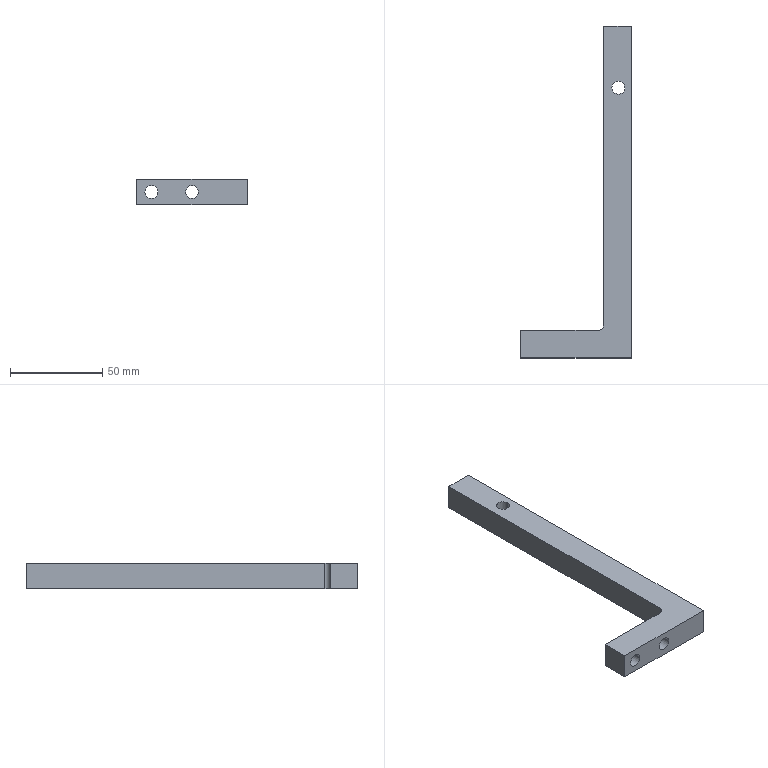Part | SolidWorks | features Cut 1, Extrusion 1, Fillet 1, ICE 1 | 1 solid | 15 faces | box 60 x 180 x 14 mm | volume 45584 mm3 | plane 8 | cylinder 7 | commonest cylinder face diameters 7 x6 6 x1
STEP:
#1=CARTESIAN_POINT('',(-10.5,146.5,7.));
#2=VERTEX_POINT('',#1);
#3=CARTESIAN_POINT('',(-3.5,146.5,7.));
#4=VERTEX_POINT('',#3);
#5=CARTESIAN_POINT('',(-7.,146.5,7.));
#6=DIRECTION('',(0.,0.,1.));
#7=DIRECTION('',(-1.,0.,0.));
#8=AXIS2_PLACEMENT_3D('',#5,#6,#7);
#9=CIRCLE('',#8,3.5);
#10=EDGE_CURVE('',#2,#4,#9,.T.);
#11=ORIENTED_EDGE('',*,*,#10,.T.);
#12=CARTESIAN_POINT('',(-3.5,146.5,-7.));
#13=VERTEX_POINT('',#12);
#14=CARTESIAN_POINT('',(-3.5,146.5,7.001));
#15=DIRECTION('',(0.,0.,-1.));
#16=VECTOR('',#15,1000.);
#17=LINE('',#14,#16);
#18=EDGE_CURVE('',#4,#13,#17,.T.);
#19=ORIENTED_EDGE('',*,*,#18,.T.);
#20=CARTESIAN_POINT('',(-10.5,146.5,-7.));
#21=VERTEX_POINT('',#20);
#22=CARTESIAN_POINT('',(-7.,146.5,-7.));
#23=DIRECTION('',(0.,0.,-1.));
#24=DIRECTION('',(-1.,0.,0.));
#25=AXIS2_PLACEMENT_3D('',#22,#23,#24);
#26=CIRCLE('',#25,3.5);
#27=EDGE_CURVE('',#13,#21,#26,.T.);
#28=ORIENTED_EDGE('',*,*,#27,.T.);
#29=CARTESIAN_POINT('',(-10.5,146.5,7.001));
#30=DIRECTION('',(0.,0.,-1.));
#31=VECTOR('',#30,1000.);
#32=LINE('',#29,#31);
#33=EDGE_CURVE('',#2,#21,#32,.T.);
#34=ORIENTED_EDGE('',*,*,#33,.F.);
#35=EDGE_LOOP('',(#11,#19,#28,#34));
#36=FACE_OUTER_BOUND('',#35,.T.);
#37=CARTESIAN_POINT('',(-7.,146.5,7.001));
#38=DIRECTION('',(0.,0.,-1.));
#39=DIRECTION('',(-1.,0.,0.));
#40=AXIS2_PLACEMENT_3D('',#37,#38,#39);
#41=CYLINDRICAL_SURFACE('',#40,3.5);
#42=ADVANCED_FACE('',(#36),#41,.F.);
#43=CARTESIAN_POINT('',(-55.5,0.,0.));
#44=VERTEX_POINT('',#43);
#45=CARTESIAN_POINT('',(-48.5,0.,0.));
#46=VERTEX_POINT('',#45);
#47=CARTESIAN_POINT('',(-52.,0.,0.));
#48=DIRECTION('',(0.,-1.,0.));
#49=DIRECTION('',(0.,0.,1.));
#50=AXIS2_PLACEMENT_3D('',#47,#48,#49);
#51=CIRCLE('',#50,3.5);
#52=EDGE_CURVE('',#44,#46,#51,.T.);
#53=ORIENTED_EDGE('',*,*,#52,.T.);
#54=CARTESIAN_POINT('',(-48.5,15.,0.));
#55=VERTEX_POINT('',#54);
#56=CARTESIAN_POINT('',(-48.5,-0.001,0.));
#57=DIRECTION('',(0.,1.,0.));
#58=VECTOR('',#57,1000.);
#59=LINE('',#56,#58);
#60=EDGE_CURVE('',#46,#55,#59,.T.);
#61=ORIENTED_EDGE('',*,*,#60,.T.);
#62=CARTESIAN_POINT('',(-55.5,15.,0.));
#63=VERTEX_POINT('',#62);
#64=CARTESIAN_POINT('',(-52.,15.,0.));
#65=DIRECTION('',(0.,1.,0.));
#66=DIRECTION('',(-1.,0.,0.));
#67=AXIS2_PLACEMENT_3D('',#64,#65,#66);
#68=CIRCLE('',#67,3.5);
#69=EDGE_CURVE('',#55,#63,#68,.T.);
#70=ORIENTED_EDGE('',*,*,#69,.T.);
#71=CARTESIAN_POINT('',(-55.5,-0.001,0.));
#72=DIRECTION('',(0.,1.,0.));
#73=VECTOR('',#72,1000.);
#74=LINE('',#71,#73);
#75=EDGE_CURVE('',#44,#63,#74,.T.);
#76=ORIENTED_EDGE('',*,*,#75,.F.);
#77=EDGE_LOOP('',(#53,#61,#70,#76));
#78=FACE_OUTER_BOUND('',#77,.T.);
#79=CARTESIAN_POINT('',(-52.,-0.001,0.));
#80=DIRECTION('',(0.,1.,0.));
#81=DIRECTION('',(-1.,0.,0.));
#82=AXIS2_PLACEMENT_3D('',#79,#80,#81);
#83=CYLINDRICAL_SURFACE('',#82,3.5);
#84=ADVANCED_FACE('',(#78),#83,.F.);
#85=CARTESIAN_POINT('',(-33.5,0.,0.));
#86=VERTEX_POINT('',#85);
#87=CARTESIAN_POINT('',(-26.5,0.,0.));
#88=VERTEX_POINT('',#87);
#89=CARTESIAN_POINT('',(-30.,0.,0.));
#90=DIRECTION('',(0.,-1.,0.));
#91=DIRECTION('',(0.,0.,1.));
#92=AXIS2_PLACEMENT_3D('',#89,#90,#91);
#93=CIRCLE('',#92,3.5);
#94=EDGE_CURVE('',#86,#88,#93,.T.);
#95=ORIENTED_EDGE('',*,*,#94,.T.);
#96=CARTESIAN_POINT('',(-26.5,15.,0.));
#97=VERTEX_POINT('',#96);
#98=CARTESIAN_POINT('',(-26.5,-0.001,0.));
#99=DIRECTION('',(0.,1.,0.));
#100=VECTOR('',#99,1000.);
#101=LINE('',#98,#100);
#102=EDGE_CURVE('',#88,#97,#101,.T.);
#103=ORIENTED_EDGE('',*,*,#102,.T.);
#104=CARTESIAN_POINT('',(-33.5,15.,0.));
#105=VERTEX_POINT('',#104);
#106=CARTESIAN_POINT('',(-30.,15.,0.));
#107=DIRECTION('',(0.,1.,0.));
#108=DIRECTION('',(-1.,0.,0.));
#109=AXIS2_PLACEMENT_3D('',#106,#107,#108);
#110=CIRCLE('',#109,3.5);
#111=EDGE_CURVE('',#97,#105,#110,.T.);
#112=ORIENTED_EDGE('',*,*,#111,.T.);
#113=CARTESIAN_POINT('',(-33.5,-0.001,0.));
#114=DIRECTION('',(0.,1.,0.));
#115=VECTOR('',#114,1000.);
#116=LINE('',#113,#115);
#117=EDGE_CURVE('',#86,#105,#116,.T.);
#118=ORIENTED_EDGE('',*,*,#117,.F.);
#119=EDGE_LOOP('',(#95,#103,#112,#118));
#120=FACE_OUTER_BOUND('',#119,.T.);
#121=CARTESIAN_POINT('',(-30.,-0.001,0.));
#122=DIRECTION('',(0.,1.,0.));
#123=DIRECTION('',(-1.,0.,0.));
#124=AXIS2_PLACEMENT_3D('',#121,#122,#123);
#125=CYLINDRICAL_SURFACE('',#124,3.5);
#126=ADVANCED_FACE('',(#120),#125,.F.);
#127=CARTESIAN_POINT('',(0.,0.,-7.));
#128=VERTEX_POINT('',#127);
#129=CARTESIAN_POINT('',(0.,180.,-7.));
#130=VERTEX_POINT('',#129);
#131=CARTESIAN_POINT('',(0.,180.,-7.));
#132=DIRECTION('',(0.,1.,0.));
#133=VECTOR('',#132,1000.);
#134=LINE('',#131,#133);
#135=EDGE_CURVE('',#128,#130,#134,.T.);
#136=ORIENTED_EDGE('',*,*,#135,.T.);
#137=CARTESIAN_POINT('',(0.,180.,7.));
#138=VERTEX_POINT('',#137);
#139=CARTESIAN_POINT('',(0.,180.,7.));
#140=DIRECTION('',(0.,0.,-1.));
#141=VECTOR('',#140,1000.);
#142=LINE('',#139,#141);
#143=EDGE_CURVE('',#138,#130,#142,.T.);
#144=ORIENTED_EDGE('',*,*,#143,.F.);
#145=CARTESIAN_POINT('',(0.,0.,7.));
#146=VERTEX_POINT('',#145);
#147=CARTESIAN_POINT('',(0.,180.,7.));
#148=DIRECTION('',(0.,1.,0.));
#149=VECTOR('',#148,1000.);
#150=LINE('',#147,#149);
#151=EDGE_CURVE('',#146,#138,#150,.T.);
#152=ORIENTED_EDGE('',*,*,#151,.F.);
#153=CARTESIAN_POINT('',(0.,0.,7.));
#154=DIRECTION('',(0.,0.,-1.));
#155=VECTOR('',#154,1000.);
#156=LINE('',#153,#155);
#157=EDGE_CURVE('',#146,#128,#156,.T.);
#158=ORIENTED_EDGE('',*,*,#157,.T.);
#159=EDGE_LOOP('',(#136,#144,#152,#158));
#160=FACE_OUTER_BOUND('',#159,.T.);
#161=CARTESIAN_POINT('',(0.,180.,7.));
#162=DIRECTION('',(-1.,0.,0.));
#163=DIRECTION('',(0.,-1.,0.));
#164=AXIS2_PLACEMENT_3D('',#161,#162,#163);
#165=PLANE('',#164);
#166=ADVANCED_FACE('',(#160),#165,.F.);
#167=CARTESIAN_POINT('',(-15.,180.,-7.));
#168=VERTEX_POINT('',#167);
#169=CARTESIAN_POINT('',(0.,180.,-7.));
#170=DIRECTION('',(-1.,0.,0.));
#171=VECTOR('',#170,1000.);
#172=LINE('',#169,#171);
#173=EDGE_CURVE('',#130,#168,#172,.T.);
#174=ORIENTED_EDGE('',*,*,#173,.T.);
#175=CARTESIAN_POINT('',(-15.,180.,7.));
#176=VERTEX_POINT('',#175);
#177=CARTESIAN_POINT('',(-15.,180.,7.));
#178=DIRECTION('',(0.,0.,-1.));
#179=VECTOR('',#178,1000.);
#180=LINE('',#177,#179);
#181=EDGE_CURVE('',#176,#168,#180,.T.);
#182=ORIENTED_EDGE('',*,*,#181,.F.);
#183=CARTESIAN_POINT('',(0.,180.,7.));
#184=DIRECTION('',(-1.,0.,0.));
#185=VECTOR('',#184,1000.);
#186=LINE('',#183,#185);
#187=EDGE_CURVE('',#138,#176,#186,.T.);
#188=ORIENTED_EDGE('',*,*,#187,.F.);
#189=ORIENTED_EDGE('',*,*,#143,.T.);
#190=EDGE_LOOP('',(#174,#182,#188,#189));
#191=FACE_OUTER_BOUND('',#190,.T.);
#192=CARTESIAN_POINT('',(0.,180.,7.));
#193=DIRECTION('',(0.,-1.,0.));
#194=DIRECTION('',(0.,0.,-1.));
#195=AXIS2_PLACEMENT_3D('',#192,#193,#194);
#196=PLANE('',#195);
#197=ADVANCED_FACE('',(#191),#196,.F.);
#198=CARTESIAN_POINT('',(-15.,18.,-7.));
#199=VERTEX_POINT('',#198);
#200=CARTESIAN_POINT('',(-15.,180.,-7.));
#201=DIRECTION('',(0.,-1.,0.));
#202=VECTOR('',#201,1000.);
#203=LINE('',#200,#202);
#204=EDGE_CURVE('',#168,#199,#203,.T.);
#205=ORIENTED_EDGE('',*,*,#204,.T.);
#206=CARTESIAN_POINT('',(-15.,18.,7.));
#207=VERTEX_POINT('',#206);
#208=CARTESIAN_POINT('',(-15.,18.,7.));
#209=DIRECTION('',(0.,0.,1.));
#210=VECTOR('',#209,1000.);
#211=LINE('',#208,#210);
#212=EDGE_CURVE('',#199,#207,#211,.T.);
#213=ORIENTED_EDGE('',*,*,#212,.T.);
#214=CARTESIAN_POINT('',(-15.,180.,7.));
#215=DIRECTION('',(0.,-1.,0.));
#216=VECTOR('',#215,1000.);
#217=LINE('',#214,#216);
#218=EDGE_CURVE('',#176,#207,#217,.T.);
#219=ORIENTED_EDGE('',*,*,#218,.F.);
#220=ORIENTED_EDGE('',*,*,#181,.T.);
#221=EDGE_LOOP('',(#205,#213,#219,#220));
#222=FACE_OUTER_BOUND('',#221,.T.);
#223=CARTESIAN_POINT('',(-15.,180.,7.));
#224=DIRECTION('',(1.,0.,0.));
#225=DIRECTION('',(0.,1.,0.));
#226=AXIS2_PLACEMENT_3D('',#223,#224,#225);
#227=PLANE('',#226);
#228=ADVANCED_FACE('',(#222),#227,.F.);
#229=CARTESIAN_POINT('',(-52.,15.,0.));
#230=DIRECTION('',(0.,1.,0.));
#231=DIRECTION('',(-1.,0.,0.));
#232=AXIS2_PLACEMENT_3D('',#229,#230,#231);
#233=CIRCLE('',#232,3.5);
#234=EDGE_CURVE('',#63,#55,#233,.T.);
#235=ORIENTED_EDGE('',*,*,#234,.F.);
#236=ORIENTED_EDGE('',*,*,#69,.F.);
#237=EDGE_LOOP('',(#235,#236));
#238=FACE_BOUND('',#237,.T.);
#239=CARTESIAN_POINT('',(-30.,15.,0.));
#240=DIRECTION('',(0.,1.,0.));
#241=DIRECTION('',(-1.,0.,0.));
#242=AXIS2_PLACEMENT_3D('',#239,#240,#241);
#243=CIRCLE('',#242,3.5);
#244=EDGE_CURVE('',#105,#97,#243,.T.);
#245=ORIENTED_EDGE('',*,*,#244,.F.);
#246=ORIENTED_EDGE('',*,*,#111,.F.);
#247=EDGE_LOOP('',(#245,#246));
#248=FACE_BOUND('',#247,.T.);
#249=CARTESIAN_POINT('',(-18.,15.,7.));
#250=VERTEX_POINT('',#249);
#251=CARTESIAN_POINT('',(-60.,15.,7.));
#252=VERTEX_POINT('',#251);
#253=CARTESIAN_POINT('',(-15.,15.,7.));
#254=DIRECTION('',(-1.,0.,0.));
#255=VECTOR('',#254,1000.);
#256=LINE('',#253,#255);
#257=EDGE_CURVE('',#250,#252,#256,.T.);
#258=ORIENTED_EDGE('',*,*,#257,.F.);
#259=CARTESIAN_POINT('',(-18.,15.,-7.));
#260=VERTEX_POINT('',#259);
#261=CARTESIAN_POINT('',(-18.,15.,-7.));
#262=DIRECTION('',(0.,0.,-1.));
#263=VECTOR('',#262,1000.);
#264=LINE('',#261,#263);
#265=EDGE_CURVE('',#250,#260,#264,.T.);
#266=ORIENTED_EDGE('',*,*,#265,.T.);
#267=CARTESIAN_POINT('',(-60.,15.,-7.));
#268=VERTEX_POINT('',#267);
#269=CARTESIAN_POINT('',(-15.,15.,-7.));
#270=DIRECTION('',(-1.,0.,0.));
#271=VECTOR('',#270,1000.);
#272=LINE('',#269,#271);
#273=EDGE_CURVE('',#260,#268,#272,.T.);
#274=ORIENTED_EDGE('',*,*,#273,.T.);
#275=CARTESIAN_POINT('',(-60.,15.,7.));
#276=DIRECTION('',(0.,0.,-1.));
#277=VECTOR('',#276,1000.);
#278=LINE('',#275,#277);
#279=EDGE_CURVE('',#252,#268,#278,.T.);
#280=ORIENTED_EDGE('',*,*,#279,.F.);
#281=EDGE_LOOP('',(#258,#266,#274,#280));
#282=FACE_OUTER_BOUND('',#281,.T.);
#283=CARTESIAN_POINT('',(-15.,15.,7.));
#284=DIRECTION('',(0.,-1.,0.));
#285=DIRECTION('',(1.,0.,0.));
#286=AXIS2_PLACEMENT_3D('',#283,#284,#285);
#287=PLANE('',#286);
#288=ADVANCED_FACE('',(#238,#248,#282),#287,.F.);
#289=CARTESIAN_POINT('',(-60.,0.,-7.));
#290=VERTEX_POINT('',#289);
#291=CARTESIAN_POINT('',(-60.,15.,-7.));
#292=DIRECTION('',(0.,-1.,0.));
#293=VECTOR('',#292,1000.);
#294=LINE('',#291,#293);
#295=EDGE_CURVE('',#268,#290,#294,.T.);
#296=ORIENTED_EDGE('',*,*,#295,.T.);
#297=CARTESIAN_POINT('',(-60.,0.,7.));
#298=VERTEX_POINT('',#297);
#299=CARTESIAN_POINT('',(-60.,0.,7.));
#300=DIRECTION('',(0.,0.,-1.));
#301=VECTOR('',#300,1000.);
#302=LINE('',#299,#301);
#303=EDGE_CURVE('',#298,#290,#302,.T.);
#304=ORIENTED_EDGE('',*,*,#303,.F.);
#305=CARTESIAN_POINT('',(-60.,15.,7.));
#306=DIRECTION('',(0.,-1.,0.));
#307=VECTOR('',#306,1000.);
#308=LINE('',#305,#307);
#309=EDGE_CURVE('',#252,#298,#308,.T.);
#310=ORIENTED_EDGE('',*,*,#309,.F.);
#311=ORIENTED_EDGE('',*,*,#279,.T.);
#312=EDGE_LOOP('',(#296,#304,#310,#311));
#313=FACE_OUTER_BOUND('',#312,.T.);
#314=CARTESIAN_POINT('',(-60.,15.,7.));
#315=DIRECTION('',(1.,0.,0.));
#316=DIRECTION('',(0.,1.,0.));
#317=AXIS2_PLACEMENT_3D('',#314,#315,#316);
#318=PLANE('',#317);
#319=ADVANCED_FACE('',(#313),#318,.F.);
#320=ORIENTED_EDGE('',*,*,#52,.F.);
#321=CARTESIAN_POINT('',(-52.,0.,0.));
#322=DIRECTION('',(0.,-1.,0.));
#323=DIRECTION('',(0.,0.,1.));
#324=AXIS2_PLACEMENT_3D('',#321,#322,#323);
#325=CIRCLE('',#324,3.5);
#326=EDGE_CURVE('',#46,#44,#325,.T.);
#327=ORIENTED_EDGE('',*,*,#326,.F.);
#328=EDGE_LOOP('',(#320,#327));
#329=FACE_BOUND('',#328,.T.);
#330=ORIENTED_EDGE('',*,*,#94,.F.);
#331=CARTESIAN_POINT('',(-30.,0.,0.));
#332=DIRECTION('',(0.,-1.,0.));
#333=DIRECTION('',(0.,0.,1.));
#334=AXIS2_PLACEMENT_3D('',#331,#332,#333);
#335=CIRCLE('',#334,3.5);
#336=EDGE_CURVE('',#88,#86,#335,.T.);
#337=ORIENTED_EDGE('',*,*,#336,.F.);
#338=EDGE_LOOP('',(#330,#337));
#339=FACE_BOUND('',#338,.T.);
#340=CARTESIAN_POINT('',(0.,0.,-7.));
#341=DIRECTION('',(1.,0.,0.));
#342=VECTOR('',#341,1000.);
#343=LINE('',#340,#342);
#344=EDGE_CURVE('',#290,#128,#343,.T.);
#345=ORIENTED_EDGE('',*,*,#344,.T.);
#346=ORIENTED_EDGE('',*,*,#157,.F.);
#347=CARTESIAN_POINT('',(0.,0.,7.));
#348=DIRECTION('',(1.,0.,0.));
#349=VECTOR('',#348,1000.);
#350=LINE('',#347,#349);
#351=EDGE_CURVE('',#298,#146,#350,.T.);
#352=ORIENTED_EDGE('',*,*,#351,.F.);
#353=ORIENTED_EDGE('',*,*,#303,.T.);
#354=EDGE_LOOP('',(#345,#346,#352,#353));
#355=FACE_OUTER_BOUND('',#354,.T.);
#356=CARTESIAN_POINT('',(0.,0.,7.));
#357=DIRECTION('',(0.,1.,0.));
#358=DIRECTION('',(0.,0.,1.));
#359=AXIS2_PLACEMENT_3D('',#356,#357,#358);
#360=PLANE('',#359);
#361=ADVANCED_FACE('',(#329,#339,#355),#360,.F.);
#362=ORIENTED_EDGE('',*,*,#10,.F.);
#363=CARTESIAN_POINT('',(-7.,146.5,7.));
#364=DIRECTION('',(0.,0.,1.));
#365=DIRECTION('',(-1.,0.,0.));
#366=AXIS2_PLACEMENT_3D('',#363,#364,#365);
#367=CIRCLE('',#366,3.5);
#368=EDGE_CURVE('',#4,#2,#367,.T.);
#369=ORIENTED_EDGE('',*,*,#368,.F.);
#370=EDGE_LOOP('',(#362,#369));
#371=FACE_BOUND('',#370,.T.);
#372=ORIENTED_EDGE('',*,*,#151,.T.);
#373=ORIENTED_EDGE('',*,*,#187,.T.);
#374=ORIENTED_EDGE('',*,*,#218,.T.);
#375=CARTESIAN_POINT('',(-18.,18.,7.));
#376=DIRECTION('',(0.,0.,-1.));
#377=DIRECTION('',(-1.,0.,0.));
#378=AXIS2_PLACEMENT_3D('',#375,#376,#377);
#379=CIRCLE('',#378,3.);
#380=EDGE_CURVE('',#207,#250,#379,.T.);
#381=ORIENTED_EDGE('',*,*,#380,.T.);
#382=ORIENTED_EDGE('',*,*,#257,.T.);
#383=ORIENTED_EDGE('',*,*,#309,.T.);
#384=ORIENTED_EDGE('',*,*,#351,.T.);
#385=EDGE_LOOP('',(#372,#373,#374,#381,#382,#383,#384));
#386=FACE_OUTER_BOUND('',#385,.T.);
#387=CARTESIAN_POINT('',(0.,0.,7.));
#388=DIRECTION('',(0.,0.,-1.));
#389=DIRECTION('',(-1.,0.,0.));
#390=AXIS2_PLACEMENT_3D('',#387,#388,#389);
#391=PLANE('',#390);
#392=ADVANCED_FACE('',(#371,#386),#391,.F.);
#393=CARTESIAN_POINT('',(-7.,146.5,-7.));
#394=DIRECTION('',(0.,0.,-1.));
#395=DIRECTION('',(-1.,0.,0.));
#396=AXIS2_PLACEMENT_3D('',#393,#394,#395);
#397=CIRCLE('',#396,3.5);
#398=EDGE_CURVE('',#21,#13,#397,.T.);
#399=ORIENTED_EDGE('',*,*,#398,.F.);
#400=ORIENTED_EDGE('',*,*,#27,.F.);
#401=EDGE_LOOP('',(#399,#400));
#402=FACE_BOUND('',#401,.T.);
#403=ORIENTED_EDGE('',*,*,#135,.F.);
#404=ORIENTED_EDGE('',*,*,#344,.F.);
#405=ORIENTED_EDGE('',*,*,#295,.F.);
#406=ORIENTED_EDGE('',*,*,#273,.F.);
#407=CARTESIAN_POINT('',(-18.,18.,-7.));
#408=DIRECTION('',(0.,0.,1.));
#409=DIRECTION('',(-1.,0.,0.));
#410=AXIS2_PLACEMENT_3D('',#407,#408,#409);
#411=CIRCLE('',#410,3.);
#412=EDGE_CURVE('',#260,#199,#411,.T.);
#413=ORIENTED_EDGE('',*,*,#412,.T.);
#414=ORIENTED_EDGE('',*,*,#204,.F.);
#415=ORIENTED_EDGE('',*,*,#173,.F.);
#416=EDGE_LOOP('',(#403,#404,#405,#406,#413,#414,#415));
#417=FACE_OUTER_BOUND('',#416,.T.);
#418=CARTESIAN_POINT('',(0.,0.,-7.));
#419=DIRECTION('',(0.,0.,-1.));
#420=DIRECTION('',(-1.,0.,0.));
#421=AXIS2_PLACEMENT_3D('',#418,#419,#420);
#422=PLANE('',#421);
#423=ADVANCED_FACE('',(#402,#417),#422,.T.);
#424=ORIENTED_EDGE('',*,*,#380,.F.);
#425=ORIENTED_EDGE('',*,*,#212,.F.);
#426=ORIENTED_EDGE('',*,*,#412,.F.);
#427=ORIENTED_EDGE('',*,*,#265,.F.);
#428=EDGE_LOOP('',(#424,#425,#426,#427));
#429=FACE_OUTER_BOUND('',#428,.T.);
#430=CARTESIAN_POINT('',(-18.,18.,7.));
#431=DIRECTION('',(0.,0.,1.));
#432=DIRECTION('',(1.,0.,0.));
#433=AXIS2_PLACEMENT_3D('',#430,#431,#432);
#434=CYLINDRICAL_SURFACE('',#433,3.);
#435=ADVANCED_FACE('',(#429),#434,.F.);
#436=ORIENTED_EDGE('',*,*,#102,.F.);
#437=ORIENTED_EDGE('',*,*,#336,.T.);
#438=ORIENTED_EDGE('',*,*,#117,.T.);
#439=ORIENTED_EDGE('',*,*,#244,.T.);
#440=EDGE_LOOP('',(#436,#437,#438,#439));
#441=FACE_OUTER_BOUND('',#440,.T.);
#442=CARTESIAN_POINT('',(-30.,-0.001,0.));
#443=DIRECTION('',(0.,1.,0.));
#444=DIRECTION('',(-1.,0.,0.));
#445=AXIS2_PLACEMENT_3D('',#442,#443,#444);
#446=CYLINDRICAL_SURFACE('',#445,3.5);
#447=ADVANCED_FACE('',(#441),#446,.F.);
#448=ORIENTED_EDGE('',*,*,#60,.F.);
#449=ORIENTED_EDGE('',*,*,#326,.T.);
#450=ORIENTED_EDGE('',*,*,#75,.T.);
#451=ORIENTED_EDGE('',*,*,#234,.T.);
#452=EDGE_LOOP('',(#448,#449,#450,#451));
#453=FACE_OUTER_BOUND('',#452,.T.);
#454=CARTESIAN_POINT('',(-52.,-0.001,0.));
#455=DIRECTION('',(0.,1.,0.));
#456=DIRECTION('',(-1.,0.,0.));
#457=AXIS2_PLACEMENT_3D('',#454,#455,#456);
#458=CYLINDRICAL_SURFACE('',#457,3.5);
#459=ADVANCED_FACE('',(#453),#458,.F.);
#460=ORIENTED_EDGE('',*,*,#18,.F.);
#461=ORIENTED_EDGE('',*,*,#368,.T.);
#462=ORIENTED_EDGE('',*,*,#33,.T.);
#463=ORIENTED_EDGE('',*,*,#398,.T.);
#464=EDGE_LOOP('',(#460,#461,#462,#463));
#465=FACE_OUTER_BOUND('',#464,.T.);
#466=CARTESIAN_POINT('',(-7.,146.5,7.001));
#467=DIRECTION('',(0.,0.,-1.));
#468=DIRECTION('',(-1.,0.,0.));
#469=AXIS2_PLACEMENT_3D('',#466,#467,#468);
#470=CYLINDRICAL_SURFACE('',#469,3.5);
#471=ADVANCED_FACE('',(#465),#470,.F.);
#472=CLOSED_SHELL('',(#42,#84,#126,#166,#197,#228,#288,#319,#361,#392,#423,#435,#447,#459,#471));
#473=MANIFOLD_SOLID_BREP('',#472);
#474=CARTESIAN_POINT('',(0.,0.,0.));
#475=DIRECTION('',(0.,0.,1.));
#476=DIRECTION('',(1.,0.,0.));
#477=AXIS2_PLACEMENT_3D('',#474,#475,#476);
#478=(LENGTH_UNIT()NAMED_UNIT(*)SI_UNIT(.MILLI.,.METRE.));
#479=UNCERTAINTY_MEASURE_WITH_UNIT(LENGTH_MEASURE(0.00001),#478,'','');
#480=(NAMED_UNIT(*)PLANE_ANGLE_UNIT()SI_UNIT($,.RADIAN.));
#481=(NAMED_UNIT(*)SI_UNIT($,.STERADIAN.)SOLID_ANGLE_UNIT());
#482=(GEOMETRIC_REPRESENTATION_CONTEXT(3)GLOBAL_UNCERTAINTY_ASSIGNED_CONTEXT((#479))GLOBAL_UNIT_ASSIGNED_CONTEXT((#478,#480,#481))REPRESENTATION_CONTEXT('',''));
#483=ADVANCED_BREP_SHAPE_REPRESENTATION('',(#473,#477),#482);